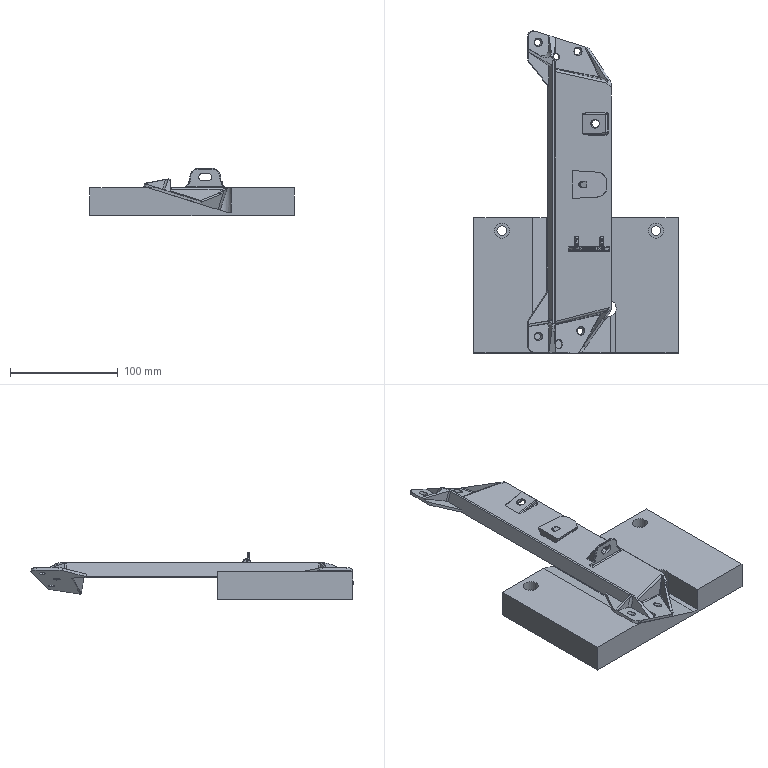Part | 2 solids | 1581 faces | box 190 x 299.709 x 43.804 mm | volume 613906 mm3 | cylinder 720 | plane 357 | spline 240 | sphere 210 | torus 42 | cone 12 | commonest cylinder face diameters 2 x435 0.6 x190 1.2 x26 1 x19 4 x13 6 x9